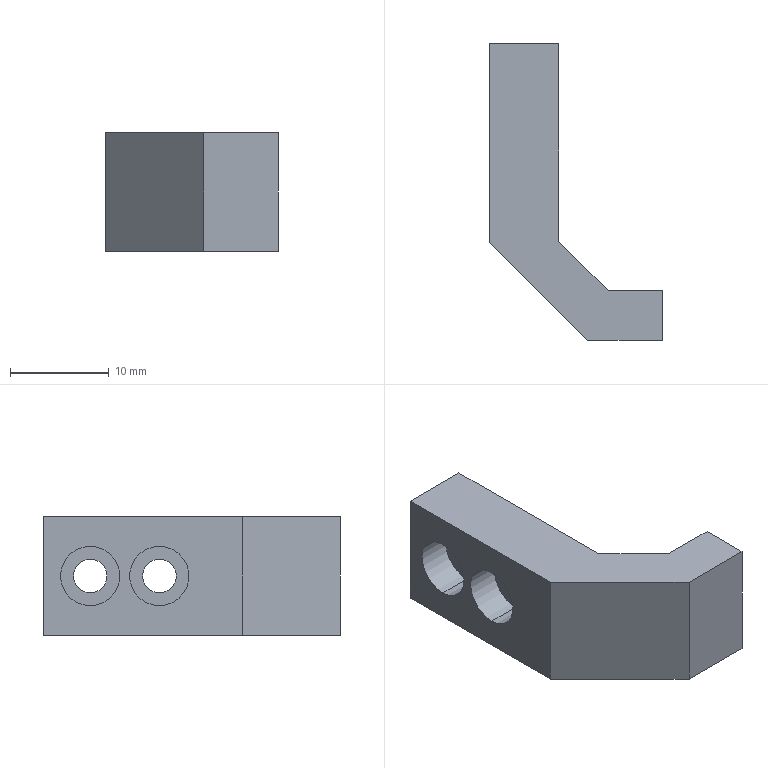Part | SolidWorks | features Extrusion 1, Fillet 1, HoleWzd 1, ICE 1 | 1 solid | 27 faces | box 17.5 x 30 x 12 mm | volume 2171 mm3 | plane 17 | cylinder 10 | commonest cylinder face diameters 3.4 x4 6 x4 4 x2
STEP:
#1=CARTESIAN_POINT('',(3.4,-4.7,-3.));
#2=VERTEX_POINT('',#1);
#3=CARTESIAN_POINT('',(3.4,-4.7,3.));
#4=VERTEX_POINT('',#3);
#5=CARTESIAN_POINT('',(3.4,-4.7,0.));
#6=DIRECTION('',(-1.,0.,0.));
#7=DIRECTION('',(0.,0.,1.));
#8=AXIS2_PLACEMENT_3D('',#5,#6,#7);
#9=CIRCLE('',#8,3.);
#10=EDGE_CURVE('',#2,#4,#9,.T.);
#11=ORIENTED_EDGE('',*,*,#10,.F.);
#12=CARTESIAN_POINT('',(0.,-4.7,-3.));
#13=VERTEX_POINT('',#12);
#14=CARTESIAN_POINT('',(0.,-4.7,-3.));
#15=DIRECTION('',(-1.,0.,0.));
#16=VECTOR('',#15,1000.);
#17=LINE('',#14,#16);
#18=EDGE_CURVE('',#2,#13,#17,.T.);
#19=ORIENTED_EDGE('',*,*,#18,.T.);
#20=CARTESIAN_POINT('',(0.,-4.7,3.));
#21=VERTEX_POINT('',#20);
#22=CARTESIAN_POINT('',(0.,-4.7,0.));
#23=DIRECTION('',(-1.,0.,0.));
#24=DIRECTION('',(0.,0.,1.));
#25=AXIS2_PLACEMENT_3D('',#22,#23,#24);
#26=CIRCLE('',#25,3.);
#27=EDGE_CURVE('',#13,#21,#26,.T.);
#28=ORIENTED_EDGE('',*,*,#27,.T.);
#29=CARTESIAN_POINT('',(0.,-4.7,3.));
#30=DIRECTION('',(-1.,0.,0.));
#31=VECTOR('',#30,1000.);
#32=LINE('',#29,#31);
#33=EDGE_CURVE('',#4,#21,#32,.T.);
#34=ORIENTED_EDGE('',*,*,#33,.F.);
#35=EDGE_LOOP('',(#11,#19,#28,#34));
#36=FACE_OUTER_BOUND('',#35,.T.);
#37=CARTESIAN_POINT('',(0.,-4.7,0.));
#38=DIRECTION('',(-1.,0.,0.));
#39=DIRECTION('',(0.,0.,1.));
#40=AXIS2_PLACEMENT_3D('',#37,#38,#39);
#41=CYLINDRICAL_SURFACE('',#40,3.);
#42=ADVANCED_FACE('',(#36),#41,.F.);
#43=CARTESIAN_POINT('',(5.,-4.7,-1.7));
#44=VERTEX_POINT('',#43);
#45=CARTESIAN_POINT('',(5.,-4.7,1.7));
#46=VERTEX_POINT('',#45);
#47=CARTESIAN_POINT('',(5.,-4.7,0.));
#48=DIRECTION('',(-1.,0.,0.));
#49=DIRECTION('',(0.,-1.,0.));
#50=AXIS2_PLACEMENT_3D('',#47,#48,#49);
#51=CIRCLE('',#50,1.7);
#52=EDGE_CURVE('',#44,#46,#51,.T.);
#53=ORIENTED_EDGE('',*,*,#52,.F.);
#54=CARTESIAN_POINT('',(3.4,-4.7,-1.7));
#55=VERTEX_POINT('',#54);
#56=CARTESIAN_POINT('',(0.,-4.7,-1.7));
#57=DIRECTION('',(-1.,0.,0.));
#58=VECTOR('',#57,1000.);
#59=LINE('',#56,#58);
#60=EDGE_CURVE('',#44,#55,#59,.T.);
#61=ORIENTED_EDGE('',*,*,#60,.T.);
#62=CARTESIAN_POINT('',(3.4,-4.7,1.7));
#63=VERTEX_POINT('',#62);
#64=CARTESIAN_POINT('',(3.4,-4.7,0.));
#65=DIRECTION('',(-1.,0.,0.));
#66=DIRECTION('',(0.,0.,1.));
#67=AXIS2_PLACEMENT_3D('',#64,#65,#66);
#68=CIRCLE('',#67,1.7);
#69=EDGE_CURVE('',#55,#63,#68,.T.);
#70=ORIENTED_EDGE('',*,*,#69,.T.);
#71=CARTESIAN_POINT('',(0.,-4.7,1.7));
#72=DIRECTION('',(-1.,0.,0.));
#73=VECTOR('',#72,1000.);
#74=LINE('',#71,#73);
#75=EDGE_CURVE('',#46,#63,#74,.T.);
#76=ORIENTED_EDGE('',*,*,#75,.F.);
#77=EDGE_LOOP('',(#53,#61,#70,#76));
#78=FACE_OUTER_BOUND('',#77,.T.);
#79=CARTESIAN_POINT('',(0.,-4.7,0.));
#80=DIRECTION('',(-1.,0.,0.));
#81=DIRECTION('',(0.,0.,1.));
#82=AXIS2_PLACEMENT_3D('',#79,#80,#81);
#83=CYLINDRICAL_SURFACE('',#82,1.7);
#84=ADVANCED_FACE('',(#78),#83,.F.);
#85=CARTESIAN_POINT('',(3.4,-11.7,-3.));
#86=VERTEX_POINT('',#85);
#87=CARTESIAN_POINT('',(3.4,-11.7,3.));
#88=VERTEX_POINT('',#87);
#89=CARTESIAN_POINT('',(3.4,-11.7,0.));
#90=DIRECTION('',(-1.,0.,0.));
#91=DIRECTION('',(0.,0.,1.));
#92=AXIS2_PLACEMENT_3D('',#89,#90,#91);
#93=CIRCLE('',#92,3.);
#94=EDGE_CURVE('',#86,#88,#93,.T.);
#95=ORIENTED_EDGE('',*,*,#94,.F.);
#96=CARTESIAN_POINT('',(0.,-11.7,-3.));
#97=VERTEX_POINT('',#96);
#98=CARTESIAN_POINT('',(0.,-11.7,-3.));
#99=DIRECTION('',(-1.,0.,0.));
#100=VECTOR('',#99,1000.);
#101=LINE('',#98,#100);
#102=EDGE_CURVE('',#86,#97,#101,.T.);
#103=ORIENTED_EDGE('',*,*,#102,.T.);
#104=CARTESIAN_POINT('',(0.,-11.7,3.));
#105=VERTEX_POINT('',#104);
#106=CARTESIAN_POINT('',(0.,-11.7,0.));
#107=DIRECTION('',(-1.,0.,0.));
#108=DIRECTION('',(0.,0.,1.));
#109=AXIS2_PLACEMENT_3D('',#106,#107,#108);
#110=CIRCLE('',#109,3.);
#111=EDGE_CURVE('',#97,#105,#110,.T.);
#112=ORIENTED_EDGE('',*,*,#111,.T.);
#113=CARTESIAN_POINT('',(0.,-11.7,3.));
#114=DIRECTION('',(-1.,0.,0.));
#115=VECTOR('',#114,1000.);
#116=LINE('',#113,#115);
#117=EDGE_CURVE('',#88,#105,#116,.T.);
#118=ORIENTED_EDGE('',*,*,#117,.F.);
#119=EDGE_LOOP('',(#95,#103,#112,#118));
#120=FACE_OUTER_BOUND('',#119,.T.);
#121=CARTESIAN_POINT('',(0.,-11.7,0.));
#122=DIRECTION('',(-1.,0.,0.));
#123=DIRECTION('',(0.,0.,1.));
#124=AXIS2_PLACEMENT_3D('',#121,#122,#123);
#125=CYLINDRICAL_SURFACE('',#124,3.);
#126=ADVANCED_FACE('',(#120),#125,.F.);
#127=CARTESIAN_POINT('',(5.,-11.7,-1.7));
#128=VERTEX_POINT('',#127);
#129=CARTESIAN_POINT('',(5.,-11.7,1.7));
#130=VERTEX_POINT('',#129);
#131=CARTESIAN_POINT('',(5.,-11.7,0.));
#132=DIRECTION('',(-1.,0.,0.));
#133=DIRECTION('',(0.,-1.,0.));
#134=AXIS2_PLACEMENT_3D('',#131,#132,#133);
#135=CIRCLE('',#134,1.7);
#136=EDGE_CURVE('',#128,#130,#135,.T.);
#137=ORIENTED_EDGE('',*,*,#136,.F.);
#138=CARTESIAN_POINT('',(3.4,-11.7,-1.7));
#139=VERTEX_POINT('',#138);
#140=CARTESIAN_POINT('',(0.,-11.7,-1.7));
#141=DIRECTION('',(-1.,0.,0.));
#142=VECTOR('',#141,1000.);
#143=LINE('',#140,#142);
#144=EDGE_CURVE('',#128,#139,#143,.T.);
#145=ORIENTED_EDGE('',*,*,#144,.T.);
#146=CARTESIAN_POINT('',(3.4,-11.7,1.7));
#147=VERTEX_POINT('',#146);
#148=CARTESIAN_POINT('',(3.4,-11.7,0.));
#149=DIRECTION('',(-1.,0.,0.));
#150=DIRECTION('',(0.,0.,1.));
#151=AXIS2_PLACEMENT_3D('',#148,#149,#150);
#152=CIRCLE('',#151,1.7);
#153=EDGE_CURVE('',#139,#147,#152,.T.);
#154=ORIENTED_EDGE('',*,*,#153,.T.);
#155=CARTESIAN_POINT('',(0.,-11.7,1.7));
#156=DIRECTION('',(-1.,0.,0.));
#157=VECTOR('',#156,1000.);
#158=LINE('',#155,#157);
#159=EDGE_CURVE('',#130,#147,#158,.T.);
#160=ORIENTED_EDGE('',*,*,#159,.F.);
#161=EDGE_LOOP('',(#137,#145,#154,#160));
#162=FACE_OUTER_BOUND('',#161,.T.);
#163=CARTESIAN_POINT('',(0.,-11.7,0.));
#164=DIRECTION('',(-1.,0.,0.));
#165=DIRECTION('',(0.,0.,1.));
#166=AXIS2_PLACEMENT_3D('',#163,#164,#165);
#167=CYLINDRICAL_SURFACE('',#166,1.7);
#168=ADVANCED_FACE('',(#162),#167,.F.);
#169=CARTESIAN_POINT('',(7.,-20.,6.));
#170=VERTEX_POINT('',#169);
#171=CARTESIAN_POINT('',(7.,-20.,2.));
#172=VERTEX_POINT('',#171);
#173=CARTESIAN_POINT('',(7.,-20.,6.));
#174=DIRECTION('',(0.,0.,-1.));
#175=VECTOR('',#174,1000.);
#176=LINE('',#173,#175);
#177=EDGE_CURVE('',#170,#172,#176,.T.);
#178=ORIENTED_EDGE('',*,*,#177,.T.);
#179=CARTESIAN_POINT('',(7.,-18.,4.));
#180=VERTEX_POINT('',#179);
#181=CARTESIAN_POINT('',(7.,-18.,2.));
#182=DIRECTION('',(-1.,0.,0.));
#183=DIRECTION('',(0.,-1.,0.));
#184=AXIS2_PLACEMENT_3D('',#181,#182,#183);
#185=CIRCLE('',#184,2.);
#186=EDGE_CURVE('',#172,#180,#185,.T.);
#187=ORIENTED_EDGE('',*,*,#186,.T.);
#188=CARTESIAN_POINT('',(7.,0.,4.));
#189=VERTEX_POINT('',#188);
#190=CARTESIAN_POINT('',(7.,-20.,4.));
#191=DIRECTION('',(0.,1.,0.));
#192=VECTOR('',#191,1000.);
#193=LINE('',#190,#192);
#194=EDGE_CURVE('',#180,#189,#193,.T.);
#195=ORIENTED_EDGE('',*,*,#194,.T.);
#196=CARTESIAN_POINT('',(7.,0.,6.));
#197=VERTEX_POINT('',#196);
#198=CARTESIAN_POINT('',(7.,0.,6.));
#199=DIRECTION('',(0.,0.,-1.));
#200=VECTOR('',#199,1000.);
#201=LINE('',#198,#200);
#202=EDGE_CURVE('',#197,#189,#201,.T.);
#203=ORIENTED_EDGE('',*,*,#202,.F.);
#204=CARTESIAN_POINT('',(7.,-20.,6.));
#205=DIRECTION('',(0.,1.,0.));
#206=VECTOR('',#205,1000.);
#207=LINE('',#204,#206);
#208=EDGE_CURVE('',#170,#197,#207,.T.);
#209=ORIENTED_EDGE('',*,*,#208,.F.);
#210=EDGE_LOOP('',(#178,#187,#195,#203,#209));
#211=FACE_OUTER_BOUND('',#210,.T.);
#212=CARTESIAN_POINT('',(7.,-20.,6.));
#213=DIRECTION('',(-1.,0.,0.));
#214=DIRECTION('',(0.,-1.,0.));
#215=AXIS2_PLACEMENT_3D('',#212,#213,#214);
#216=PLANE('',#215);
#217=ADVANCED_FACE('',(#211),#216,.F.);
#218=ORIENTED_EDGE('',*,*,#202,.T.);
#219=CARTESIAN_POINT('',(5.,0.,4.));
#220=VERTEX_POINT('',#219);
#221=CARTESIAN_POINT('',(7.,0.,4.));
#222=DIRECTION('',(1.,0.,0.));
#223=VECTOR('',#222,1000.);
#224=LINE('',#221,#223);
#225=EDGE_CURVE('',#220,#189,#224,.T.);
#226=ORIENTED_EDGE('',*,*,#225,.F.);
#227=CARTESIAN_POINT('',(5.,0.,-4.));
#228=VERTEX_POINT('',#227);
#229=CARTESIAN_POINT('',(5.,0.,-4.));
#230=DIRECTION('',(0.,0.,1.));
#231=VECTOR('',#230,1000.);
#232=LINE('',#229,#231);
#233=EDGE_CURVE('',#228,#220,#232,.T.);
#234=ORIENTED_EDGE('',*,*,#233,.F.);
#235=CARTESIAN_POINT('',(7.,0.,-4.));
#236=VERTEX_POINT('',#235);
#237=CARTESIAN_POINT('',(7.,0.,-4.));
#238=DIRECTION('',(-1.,0.,0.));
#239=VECTOR('',#238,1000.);
#240=LINE('',#237,#239);
#241=EDGE_CURVE('',#236,#228,#240,.T.);
#242=ORIENTED_EDGE('',*,*,#241,.F.);
#243=CARTESIAN_POINT('',(7.,0.,-6.));
#244=VERTEX_POINT('',#243);
#245=CARTESIAN_POINT('',(7.,0.,6.));
#246=DIRECTION('',(0.,0.,-1.));
#247=VECTOR('',#246,1000.);
#248=LINE('',#245,#247);
#249=EDGE_CURVE('',#236,#244,#248,.T.);
#250=ORIENTED_EDGE('',*,*,#249,.T.);
#251=CARTESIAN_POINT('',(0.,0.,-6.));
#252=VERTEX_POINT('',#251);
#253=CARTESIAN_POINT('',(7.,0.,-6.));
#254=DIRECTION('',(-1.,0.,0.));
#255=VECTOR('',#254,1000.);
#256=LINE('',#253,#255);
#257=EDGE_CURVE('',#244,#252,#256,.T.);
#258=ORIENTED_EDGE('',*,*,#257,.T.);
#259=CARTESIAN_POINT('',(0.,0.,6.));
#260=VERTEX_POINT('',#259);
#261=CARTESIAN_POINT('',(0.,0.,6.));
#262=DIRECTION('',(0.,0.,-1.));
#263=VECTOR('',#262,1000.);
#264=LINE('',#261,#263);
#265=EDGE_CURVE('',#260,#252,#264,.T.);
#266=ORIENTED_EDGE('',*,*,#265,.F.);
#267=CARTESIAN_POINT('',(7.,0.,6.));
#268=DIRECTION('',(-1.,0.,0.));
#269=VECTOR('',#268,1000.);
#270=LINE('',#267,#269);
#271=EDGE_CURVE('',#197,#260,#270,.T.);
#272=ORIENTED_EDGE('',*,*,#271,.F.);
#273=EDGE_LOOP('',(#218,#226,#234,#242,#250,#258,#266,#272));
#274=FACE_OUTER_BOUND('',#273,.T.);
#275=CARTESIAN_POINT('',(7.,0.,6.));
#276=DIRECTION('',(0.,-1.,0.));
#277=DIRECTION('',(1.,0.,0.));
#278=AXIS2_PLACEMENT_3D('',#275,#276,#277);
#279=PLANE('',#278);
#280=ADVANCED_FACE('',(#274),#279,.F.);
#281=CARTESIAN_POINT('',(0.,-4.7,0.));
#282=DIRECTION('',(-1.,0.,0.));
#283=DIRECTION('',(0.,0.,1.));
#284=AXIS2_PLACEMENT_3D('',#281,#282,#283);
#285=CIRCLE('',#284,3.);
#286=EDGE_CURVE('',#21,#13,#285,.T.);
#287=ORIENTED_EDGE('',*,*,#286,.F.);
#288=ORIENTED_EDGE('',*,*,#27,.F.);
#289=EDGE_LOOP('',(#287,#288));
#290=FACE_BOUND('',#289,.T.);
#291=CARTESIAN_POINT('',(0.,-11.7,0.));
#292=DIRECTION('',(-1.,0.,0.));
#293=DIRECTION('',(0.,0.,1.));
#294=AXIS2_PLACEMENT_3D('',#291,#292,#293);
#295=CIRCLE('',#294,3.);
#296=EDGE_CURVE('',#105,#97,#295,.T.);
#297=ORIENTED_EDGE('',*,*,#296,.F.);
#298=ORIENTED_EDGE('',*,*,#111,.F.);
#299=EDGE_LOOP('',(#297,#298));
#300=FACE_BOUND('',#299,.T.);
#301=CARTESIAN_POINT('',(0.,-20.071,-6.));
#302=VERTEX_POINT('',#301);
#303=CARTESIAN_POINT('',(0.,0.,-6.));
#304=DIRECTION('',(0.,-1.,0.));
#305=VECTOR('',#304,1000.);
#306=LINE('',#303,#305);
#307=EDGE_CURVE('',#252,#302,#306,.T.);
#308=ORIENTED_EDGE('',*,*,#307,.T.);
#309=CARTESIAN_POINT('',(0.,-20.071,6.));
#310=VERTEX_POINT('',#309);
#311=CARTESIAN_POINT('',(0.,-20.071,6.));
#312=DIRECTION('',(0.,0.,-1.));
#313=VECTOR('',#312,1000.);
#314=LINE('',#311,#313);
#315=EDGE_CURVE('',#310,#302,#314,.T.);
#316=ORIENTED_EDGE('',*,*,#315,.F.);
#317=CARTESIAN_POINT('',(0.,0.,6.));
#318=DIRECTION('',(0.,-1.,0.));
#319=VECTOR('',#318,1000.);
#320=LINE('',#317,#319);
#321=EDGE_CURVE('',#260,#310,#320,.T.);
#322=ORIENTED_EDGE('',*,*,#321,.F.);
#323=ORIENTED_EDGE('',*,*,#265,.T.);
#324=EDGE_LOOP('',(#308,#316,#322,#323));
#325=FACE_OUTER_BOUND('',#324,.T.);
#326=CARTESIAN_POINT('',(0.,0.,6.));
#327=DIRECTION('',(1.,0.,0.));
#328=DIRECTION('',(0.,1.,0.));
#329=AXIS2_PLACEMENT_3D('',#326,#327,#328);
#330=PLANE('',#329);
#331=ADVANCED_FACE('',(#290,#300,#325),#330,.F.);
#332=CARTESIAN_POINT('',(9.929,-30.,-6.));
#333=VERTEX_POINT('',#332);
#334=CARTESIAN_POINT('',(0.,-20.071,-6.));
#335=DIRECTION('',(0.7071,-0.7071,0.));
#336=VECTOR('',#335,1000.);
#337=LINE('',#334,#336);
#338=EDGE_CURVE('',#302,#333,#337,.T.);
#339=ORIENTED_EDGE('',*,*,#338,.T.);
#340=CARTESIAN_POINT('',(9.929,-30.,6.));
#341=VERTEX_POINT('',#340);
#342=CARTESIAN_POINT('',(9.929,-30.,6.));
#343=DIRECTION('',(0.,0.,-1.));
#344=VECTOR('',#343,1000.);
#345=LINE('',#342,#344);
#346=EDGE_CURVE('',#341,#333,#345,.T.);
#347=ORIENTED_EDGE('',*,*,#346,.F.);
#348=CARTESIAN_POINT('',(0.,-20.071,6.));
#349=DIRECTION('',(0.7071,-0.7071,0.));
#350=VECTOR('',#349,1000.);
#351=LINE('',#348,#350);
#352=EDGE_CURVE('',#310,#341,#351,.T.);
#353=ORIENTED_EDGE('',*,*,#352,.F.);
#354=ORIENTED_EDGE('',*,*,#315,.T.);
#355=EDGE_LOOP('',(#339,#347,#353,#354));
#356=FACE_OUTER_BOUND('',#355,.T.);
#357=CARTESIAN_POINT('',(0.,-20.071,6.));
#358=DIRECTION('',(0.7071,0.7071,0.));
#359=DIRECTION('',(-0.7071,0.7071,0.));
#360=AXIS2_PLACEMENT_3D('',#357,#358,#359);
#361=PLANE('',#360);
#362=ADVANCED_FACE('',(#356),#361,.F.);
#363=CARTESIAN_POINT('',(17.5,-30.,-6.));
#364=VERTEX_POINT('',#363);
#365=CARTESIAN_POINT('',(17.5,-30.,-6.));
#366=DIRECTION('',(1.,0.,0.));
#367=VECTOR('',#366,1000.);
#368=LINE('',#365,#367);
#369=EDGE_CURVE('',#333,#364,#368,.T.);
#370=ORIENTED_EDGE('',*,*,#369,.T.);
#371=CARTESIAN_POINT('',(17.5,-30.,6.));
#372=VERTEX_POINT('',#371);
#373=CARTESIAN_POINT('',(17.5,-30.,6.));
#374=DIRECTION('',(0.,0.,-1.));
#375=VECTOR('',#374,1000.);
#376=LINE('',#373,#375);
#377=EDGE_CURVE('',#372,#364,#376,.T.);
#378=ORIENTED_EDGE('',*,*,#377,.F.);
#379=CARTESIAN_POINT('',(17.5,-30.,6.));
#380=DIRECTION('',(1.,0.,0.));
#381=VECTOR('',#380,1000.);
#382=LINE('',#379,#381);
#383=EDGE_CURVE('',#341,#372,#382,.T.);
#384=ORIENTED_EDGE('',*,*,#383,.F.);
#385=ORIENTED_EDGE('',*,*,#346,.T.);
#386=EDGE_LOOP('',(#370,#378,#384,#385));
#387=FACE_OUTER_BOUND('',#386,.T.);
#388=CARTESIAN_POINT('',(17.5,-30.,6.));
#389=DIRECTION('',(0.,1.,0.));
#390=DIRECTION('',(-1.,0.,0.));
#391=AXIS2_PLACEMENT_3D('',#388,#389,#390);
#392=PLANE('',#391);
#393=ADVANCED_FACE('',(#387),#392,.F.);
#394=CARTESIAN_POINT('',(17.5,-25.,-6.));
#395=VERTEX_POINT('',#394);
#396=CARTESIAN_POINT('',(17.5,-25.,-6.));
#397=DIRECTION('',(0.,1.,0.));
#398=VECTOR('',#397,1000.);
#399=LINE('',#396,#398);
#400=EDGE_CURVE('',#364,#395,#399,.T.);
#401=ORIENTED_EDGE('',*,*,#400,.T.);
#402=CARTESIAN_POINT('',(17.5,-25.,6.));
#403=VERTEX_POINT('',#402);
#404=CARTESIAN_POINT('',(17.5,-25.,6.));
#405=DIRECTION('',(0.,0.,-1.));
#406=VECTOR('',#405,1000.);
#407=LINE('',#404,#406);
#408=EDGE_CURVE('',#403,#395,#407,.T.);
#409=ORIENTED_EDGE('',*,*,#408,.F.);
#410=CARTESIAN_POINT('',(17.5,-25.,6.));
#411=DIRECTION('',(0.,1.,0.));
#412=VECTOR('',#411,1000.);
#413=LINE('',#410,#412);
#414=EDGE_CURVE('',#372,#403,#413,.T.);
#415=ORIENTED_EDGE('',*,*,#414,.F.);
#416=ORIENTED_EDGE('',*,*,#377,.T.);
#417=EDGE_LOOP('',(#401,#409,#415,#416));
#418=FACE_OUTER_BOUND('',#417,.T.);
#419=CARTESIAN_POINT('',(17.5,-25.,6.));
#420=DIRECTION('',(-1.,0.,0.));
#421=DIRECTION('',(0.,0.,1.));
#422=AXIS2_PLACEMENT_3D('',#419,#420,#421);
#423=PLANE('',#422);
#424=ADVANCED_FACE('',(#418),#423,.F.);
#425=CARTESIAN_POINT('',(12.,-25.,-6.));
#426=VERTEX_POINT('',#425);
#427=CARTESIAN_POINT('',(12.,-25.,-6.));
#428=DIRECTION('',(-1.,0.,0.));
#429=VECTOR('',#428,1000.);
#430=LINE('',#427,#429);
#431=EDGE_CURVE('',#395,#426,#430,.T.);
#432=ORIENTED_EDGE('',*,*,#431,.T.);
#433=CARTESIAN_POINT('',(12.,-25.,6.));
#434=VERTEX_POINT('',#433);
#435=CARTESIAN_POINT('',(12.,-25.,6.));
#436=DIRECTION('',(0.,0.,-1.));
#437=VECTOR('',#436,1000.);
#438=LINE('',#435,#437);
#439=EDGE_CURVE('',#434,#426,#438,.T.);
#440=ORIENTED_EDGE('',*,*,#439,.F.);
#441=CARTESIAN_POINT('',(12.,-25.,6.));
#442=DIRECTION('',(-1.,0.,0.));
#443=VECTOR('',#442,1000.);
#444=LINE('',#441,#443);
#445=EDGE_CURVE('',#403,#434,#444,.T.);
#446=ORIENTED_EDGE('',*,*,#445,.F.);
#447=ORIENTED_EDGE('',*,*,#408,.T.);
#448=EDGE_LOOP('',(#432,#440,#446,#447));
#449=FACE_OUTER_BOUND('',#448,.T.);
#450=CARTESIAN_POINT('',(12.,-25.,6.));
#451=DIRECTION('',(0.,-1.,0.));
#452=DIRECTION('',(1.,0.,0.));
#453=AXIS2_PLACEMENT_3D('',#450,#451,#452);
#454=PLANE('',#453);
#455=ADVANCED_FACE('',(#449),#454,.F.);
#456=CARTESIAN_POINT('',(7.,-20.,-6.));
#457=VERTEX_POINT('',#456);
#458=CARTESIAN_POINT('',(12.,-25.,-6.));
#459=DIRECTION('',(-0.7071,0.7071,0.));
#460=VECTOR('',#459,1000.);
#461=LINE('',#458,#460);
#462=EDGE_CURVE('',#426,#457,#461,.T.);
#463=ORIENTED_EDGE('',*,*,#462,.T.);
#464=CARTESIAN_POINT('',(7.,-20.,-2.));
#465=VERTEX_POINT('',#464);
#466=CARTESIAN_POINT('',(7.,-20.,6.));
#467=DIRECTION('',(0.,0.,-1.));
#468=VECTOR('',#467,1000.);
#469=LINE('',#466,#468);
#470=EDGE_CURVE('',#465,#457,#469,.T.);
#471=ORIENTED_EDGE('',*,*,#470,.F.);
#472=CARTESIAN_POINT('',(7.,-20.,-4.));
#473=DIRECTION('',(0.,0.,-1.));
#474=VECTOR('',#473,1000.);
#475=LINE('',#472,#474);
#476=EDGE_CURVE('',#172,#465,#475,.T.);
#477=ORIENTED_EDGE('',*,*,#476,.F.);
#478=ORIENTED_EDGE('',*,*,#177,.F.);
#479=CARTESIAN_POINT('',(12.,-25.,6.));
#480=DIRECTION('',(-0.7071,0.7071,0.));
#481=VECTOR('',#480,1000.);
#482=LINE('',#479,#481);
#483=EDGE_CURVE('',#434,#170,#482,.T.);
#484=ORIENTED_EDGE('',*,*,#483,.F.);
#485=ORIENTED_EDGE('',*,*,#439,.T.);
#486=EDGE_LOOP('',(#463,#471,#477,#478,#484,#485));
#487=FACE_OUTER_BOUND('',#486,.T.);
#488=CARTESIAN_POINT('',(12.,-25.,6.));
#489=DIRECTION('',(-0.7071,-0.7071,0.));
#490=DIRECTION('',(0.7071,-0.7071,0.));
#491=AXIS2_PLACEMENT_3D('',#488,#489,#490);
#492=PLANE('',#491);
#493=ADVANCED_FACE('',(#487),#492,.F.);
#494=ORIENTED_EDGE('',*,*,#249,.F.);
#495=CARTESIAN_POINT('',(7.,-18.,-4.));
#496=VERTEX_POINT('',#495);
#497=CARTESIAN_POINT('',(7.,-20.,-4.));
#498=DIRECTION('',(0.,1.,0.));
#499=VECTOR('',#498,1000.);
#500=LINE('',#497,#499);
#501=EDGE_CURVE('',#496,#236,#500,.T.);
#502=ORIENTED_EDGE('',*,*,#501,.F.);
#503=CARTESIAN_POINT('',(7.,-18.,-2.));
#504=DIRECTION('',(-1.,0.,0.));
#505=DIRECTION('',(0.,-1.,0.));
#506=AXIS2_PLACEMENT_3D('',#503,#504,#505);
#507=CIRCLE('',#506,2.);
#508=EDGE_CURVE('',#496,#465,#507,.T.);
#509=ORIENTED_EDGE('',*,*,#508,.T.);
#510=ORIENTED_EDGE('',*,*,#470,.T.);
#511=CARTESIAN_POINT('',(7.,-20.,-6.));
#512=DIRECTION('',(0.,1.,0.));
#513=VECTOR('',#512,1000.);
#514=LINE('',#511,#513);
#515=EDGE_CURVE('',#457,#244,#514,.T.);
#516=ORIENTED_EDGE('',*,*,#515,.T.);
#517=EDGE_LOOP('',(#494,#502,#509,#510,#516));
#518=FACE_OUTER_BOUND('',#517,.T.);
#519=CARTESIAN_POINT('',(7.,-20.,6.));
#520=DIRECTION('',(-1.,0.,0.));
#521=DIRECTION('',(0.,-1.,0.));
#522=AXIS2_PLACEMENT_3D('',#519,#520,#521);
#523=PLANE('',#522);
#524=ADVANCED_FACE('',(#518),#523,.F.);
#525=ORIENTED_EDGE('',*,*,#271,.T.);
#526=ORIENTED_EDGE('',*,*,#321,.T.);
#527=ORIENTED_EDGE('',*,*,#352,.T.);
#528=ORIENTED_EDGE('',*,*,#383,.T.);
#529=ORIENTED_EDGE('',*,*,#414,.T.);
#530=ORIENTED_EDGE('',*,*,#445,.T.);
#531=ORIENTED_EDGE('',*,*,#483,.T.);
#532=ORIENTED_EDGE('',*,*,#208,.T.);
#533=EDGE_LOOP('',(#525,#526,#527,#528,#529,#530,#531,#532));
#534=FACE_OUTER_BOUND('',#533,.T.);
#535=CARTESIAN_POINT('',(0.,0.,6.));
#536=DIRECTION('',(0.,0.,1.));
#537=DIRECTION('',(1.,0.,0.));
#538=AXIS2_PLACEMENT_3D('',#535,#536,#537);
#539=PLANE('',#538);
#540=ADVANCED_FACE('',(#534),#539,.T.);
#541=ORIENTED_EDGE('',*,*,#257,.F.);
#542=ORIENTED_EDGE('',*,*,#515,.F.);
#543=ORIENTED_EDGE('',*,*,#462,.F.);
#544=ORIENTED_EDGE('',*,*,#431,.F.);
#545=ORIENTED_EDGE('',*,*,#400,.F.);
#546=ORIENTED_EDGE('',*,*,#369,.F.);
#547=ORIENTED_EDGE('',*,*,#338,.F.);
#548=ORIENTED_EDGE('',*,*,#307,.F.);
#549=EDGE_LOOP('',(#541,#542,#543,#544,#545,#546,#547,#548));
#550=FACE_OUTER_BOUND('',#549,.T.);
#551=CARTESIAN_POINT('',(0.,0.,-6.));
#552=DIRECTION('',(0.,0.,1.));
#553=DIRECTION('',(1.,0.,0.));
#554=AXIS2_PLACEMENT_3D('',#551,#552,#553);
#555=PLANE('',#554);
#556=ADVANCED_FACE('',(#550),#555,.F.);
#557=ORIENTED_EDGE('',*,*,#194,.F.);
#558=CARTESIAN_POINT('',(5.,-18.,4.));
#559=VERTEX_POINT('',#558);
#560=CARTESIAN_POINT('',(5.,-18.,4.));
#561=DIRECTION('',(-1.,0.,0.));
#562=VECTOR('',#561,1000.);
#563=LINE('',#560,#562);
#564=EDGE_CURVE('',#180,#559,#563,.T.);
#565=ORIENTED_EDGE('',*,*,#564,.T.);
#566=CARTESIAN_POINT('',(5.,-20.,4.));
#567=DIRECTION('',(0.,1.,0.));
#568=VECTOR('',#567,1000.);
#569=LINE('',#566,#568);
#570=EDGE_CURVE('',#559,#220,#569,.T.);
#571=ORIENTED_EDGE('',*,*,#570,.T.);
#572=ORIENTED_EDGE('',*,*,#225,.T.);
#573=EDGE_LOOP('',(#557,#565,#571,#572));
#574=FACE_OUTER_BOUND('',#573,.T.);
#575=CARTESIAN_POINT('',(7.,-20.,4.));
#576=DIRECTION('',(0.,0.,1.));
#577=DIRECTION('',(1.,0.,0.));
#578=AXIS2_PLACEMENT_3D('',#575,#576,#577);
#579=PLANE('',#578);
#580=ADVANCED_FACE('',(#574),#579,.F.);
#581=CARTESIAN_POINT('',(5.,-4.7,0.));
#582=DIRECTION('',(-1.,0.,0.));
#583=DIRECTION('',(0.,-1.,0.));
#584=AXIS2_PLACEMENT_3D('',#581,#582,#583);
#585=CIRCLE('',#584,1.7);
#586=EDGE_CURVE('',#46,#44,#585,.T.);
#587=ORIENTED_EDGE('',*,*,#586,.T.);
#588=ORIENTED_EDGE('',*,*,#52,.T.);
#589=EDGE_LOOP('',(#587,#588));
#590=FACE_BOUND('',#589,.T.);
#591=CARTESIAN_POINT('',(5.,-11.7,0.));
#592=DIRECTION('',(-1.,0.,0.));
#593=DIRECTION('',(0.,-1.,0.));
#594=AXIS2_PLACEMENT_3D('',#591,#592,#593);
#595=CIRCLE('',#594,1.7);
#596=EDGE_CURVE('',#130,#128,#595,.T.);
#597=ORIENTED_EDGE('',*,*,#596,.T.);
#598=ORIENTED_EDGE('',*,*,#136,.T.);
#599=EDGE_LOOP('',(#597,#598));
#600=FACE_BOUND('',#599,.T.);
#601=ORIENTED_EDGE('',*,*,#570,.F.);
#602=CARTESIAN_POINT('',(5.,-20.,2.));
#603=VERTEX_POINT('',#602);
#604=CARTESIAN_POINT('',(5.,-18.,2.));
#605=DIRECTION('',(1.,0.,0.));
#606=DIRECTION('',(0.,-1.,0.));
#607=AXIS2_PLACEMENT_3D('',#604,#605,#606);
#608=CIRCLE('',#607,2.);
#609=EDGE_CURVE('',#559,#603,#608,.T.);
#610=ORIENTED_EDGE('',*,*,#609,.T.);
#611=CARTESIAN_POINT('',(5.,-20.,-2.));
#612=VERTEX_POINT('',#611);
#613=CARTESIAN_POINT('',(5.,-20.,-4.));
#614=DIRECTION('',(0.,0.,1.));
#615=VECTOR('',#614,1000.);
#616=LINE('',#613,#615);
#617=EDGE_CURVE('',#612,#603,#616,.T.);
#618=ORIENTED_EDGE('',*,*,#617,.F.);
#619=CARTESIAN_POINT('',(5.,-18.,-4.));
#620=VERTEX_POINT('',#619);
#621=CARTESIAN_POINT('',(5.,-18.,-2.));
#622=DIRECTION('',(1.,0.,0.));
#623=DIRECTION('',(0.,-1.,0.));
#624=AXIS2_PLACEMENT_3D('',#621,#622,#623);
#625=CIRCLE('',#624,2.);
#626=EDGE_CURVE('',#612,#620,#625,.T.);
#627=ORIENTED_EDGE('',*,*,#626,.T.);
#628=CARTESIAN_POINT('',(5.,-20.,-4.));
#629=DIRECTION('',(0.,1.,0.));
#630=VECTOR('',#629,1000.);
#631=LINE('',#628,#630);
#632=EDGE_CURVE('',#620,#228,#631,.T.);
#633=ORIENTED_EDGE('',*,*,#632,.T.);
#634=ORIENTED_EDGE('',*,*,#233,.T.);
#635=EDGE_LOOP('',(#601,#610,#618,#627,#633,#634));
#636=FACE_OUTER_BOUND('',#635,.T.);
#637=CARTESIAN_POINT('',(5.,-20.,-4.));
#638=DIRECTION('',(-1.,0.,0.));
#639=DIRECTION('',(0.,-1.,0.));
#640=AXIS2_PLACEMENT_3D('',#637,#638,#639);
#641=PLANE('',#640);
#642=ADVANCED_FACE('',(#590,#600,#636),#641,.F.);
#643=ORIENTED_EDGE('',*,*,#632,.F.);
#644=CARTESIAN_POINT('',(7.,-18.,-4.));
#645=DIRECTION('',(1.,0.,0.));
#646=VECTOR('',#645,1000.);
#647=LINE('',#644,#646);
#648=EDGE_CURVE('',#620,#496,#647,.T.);
#649=ORIENTED_EDGE('',*,*,#648,.T.);
#650=ORIENTED_EDGE('',*,*,#501,.T.);
#651=ORIENTED_EDGE('',*,*,#241,.T.);
#652=EDGE_LOOP('',(#643,#649,#650,#651));
#653=FACE_OUTER_BOUND('',#652,.T.);
#654=CARTESIAN_POINT('',(7.,-20.,-4.));
#655=DIRECTION('',(0.,0.,-1.));
#656=DIRECTION('',(-1.,0.,0.));
#657=AXIS2_PLACEMENT_3D('',#654,#655,#656);
#658=PLANE('',#657);
#659=ADVANCED_FACE('',(#653),#658,.F.);
#660=ORIENTED_EDGE('',*,*,#617,.T.);
#661=CARTESIAN_POINT('',(7.,-20.,2.));
#662=DIRECTION('',(1.,0.,0.));
#663=VECTOR('',#662,1000.);
#664=LINE('',#661,#663);
#665=EDGE_CURVE('',#603,#172,#664,.T.);
#666=ORIENTED_EDGE('',*,*,#665,.T.);
#667=ORIENTED_EDGE('',*,*,#476,.T.);
#668=CARTESIAN_POINT('',(5.,-20.,-2.));
#669=DIRECTION('',(-1.,0.,0.));
#670=VECTOR('',#669,1000.);
#671=LINE('',#668,#670);
#672=EDGE_CURVE('',#465,#612,#671,.T.);
#673=ORIENTED_EDGE('',*,*,#672,.T.);
#674=EDGE_LOOP('',(#660,#666,#667,#673));
#675=FACE_OUTER_BOUND('',#674,.T.);
#676=CARTESIAN_POINT('',(0.,-20.,0.));
#677=DIRECTION('',(0.,-1.,0.));
#678=DIRECTION('',(1.,0.,0.));
#679=AXIS2_PLACEMENT_3D('',#676,#677,#678);
#680=PLANE('',#679);
#681=ADVANCED_FACE('',(#675),#680,.F.);
#682=ORIENTED_EDGE('',*,*,#609,.F.);
#683=ORIENTED_EDGE('',*,*,#564,.F.);
#684=ORIENTED_EDGE('',*,*,#186,.F.);
#685=ORIENTED_EDGE('',*,*,#665,.F.);
#686=EDGE_LOOP('',(#682,#683,#684,#685));
#687=FACE_OUTER_BOUND('',#686,.T.);
#688=CARTESIAN_POINT('',(0.,-18.,2.));
#689=DIRECTION('',(-1.,0.,0.));
#690=DIRECTION('',(0.,-1.,0.));
#691=AXIS2_PLACEMENT_3D('',#688,#689,#690);
#692=CYLINDRICAL_SURFACE('',#691,2.);
#693=ADVANCED_FACE('',(#687),#692,.F.);
#694=ORIENTED_EDGE('',*,*,#508,.F.);
#695=ORIENTED_EDGE('',*,*,#648,.F.);
#696=ORIENTED_EDGE('',*,*,#626,.F.);
#697=ORIENTED_EDGE('',*,*,#672,.F.);
#698=EDGE_LOOP('',(#694,#695,#696,#697));
#699=FACE_OUTER_BOUND('',#698,.T.);
#700=CARTESIAN_POINT('',(0.,-18.,-2.));
#701=DIRECTION('',(1.,0.,0.));
#702=DIRECTION('',(0.,1.,0.));
#703=AXIS2_PLACEMENT_3D('',#700,#701,#702);
#704=CYLINDRICAL_SURFACE('',#703,2.);
#705=ADVANCED_FACE('',(#699),#704,.F.);
#706=ORIENTED_EDGE('',*,*,#144,.F.);
#707=ORIENTED_EDGE('',*,*,#596,.F.);
#708=ORIENTED_EDGE('',*,*,#159,.T.);
#709=CARTESIAN_POINT('',(3.4,-11.7,0.));
#710=DIRECTION('',(-1.,0.,0.));
#711=DIRECTION('',(0.,0.,1.));
#712=AXIS2_PLACEMENT_3D('',#709,#710,#711);
#713=CIRCLE('',#712,1.7);
#714=EDGE_CURVE('',#147,#139,#713,.T.);
#715=ORIENTED_EDGE('',*,*,#714,.T.);
#716=EDGE_LOOP('',(#706,#707,#708,#715));
#717=FACE_OUTER_BOUND('',#716,.T.);
#718=CARTESIAN_POINT('',(0.,-11.7,0.));
#719=DIRECTION('',(-1.,0.,0.));
#720=DIRECTION('',(0.,0.,1.));
#721=AXIS2_PLACEMENT_3D('',#718,#719,#720);
#722=CYLINDRICAL_SURFACE('',#721,1.7);
#723=ADVANCED_FACE('',(#717),#722,.F.);
#724=ORIENTED_EDGE('',*,*,#714,.F.);
#725=ORIENTED_EDGE('',*,*,#153,.F.);
#726=EDGE_LOOP('',(#724,#725));
#727=FACE_BOUND('',#726,.T.);
#728=CARTESIAN_POINT('',(3.4,-11.7,0.));
#729=DIRECTION('',(-1.,0.,0.));
#730=DIRECTION('',(0.,0.,1.));
#731=AXIS2_PLACEMENT_3D('',#728,#729,#730);
#732=CIRCLE('',#731,3.);
#733=EDGE_CURVE('',#88,#86,#732,.T.);
#734=ORIENTED_EDGE('',*,*,#733,.T.);
#735=ORIENTED_EDGE('',*,*,#94,.T.);
#736=EDGE_LOOP('',(#734,#735));
#737=FACE_OUTER_BOUND('',#736,.T.);
#738=CARTESIAN_POINT('',(3.4,-10.,0.));
#739=DIRECTION('',(1.,0.,0.));
#740=DIRECTION('',(0.,0.,-1.));
#741=AXIS2_PLACEMENT_3D('',#738,#739,#740);
#742=PLANE('',#741);
#743=ADVANCED_FACE('',(#727,#737),#742,.F.);
#744=ORIENTED_EDGE('',*,*,#102,.F.);
#745=ORIENTED_EDGE('',*,*,#733,.F.);
#746=ORIENTED_EDGE('',*,*,#117,.T.);
#747=ORIENTED_EDGE('',*,*,#296,.T.);
#748=EDGE_LOOP('',(#744,#745,#746,#747));
#749=FACE_OUTER_BOUND('',#748,.T.);
#750=CARTESIAN_POINT('',(0.,-11.7,0.));
#751=DIRECTION('',(-1.,0.,0.));
#752=DIRECTION('',(0.,0.,1.));
#753=AXIS2_PLACEMENT_3D('',#750,#751,#752);
#754=CYLINDRICAL_SURFACE('',#753,3.);
#755=ADVANCED_FACE('',(#749),#754,.F.);
#756=ORIENTED_EDGE('',*,*,#60,.F.);
#757=ORIENTED_EDGE('',*,*,#586,.F.);
#758=ORIENTED_EDGE('',*,*,#75,.T.);
#759=CARTESIAN_POINT('',(3.4,-4.7,0.));
#760=DIRECTION('',(-1.,0.,0.));
#761=DIRECTION('',(0.,0.,1.));
#762=AXIS2_PLACEMENT_3D('',#759,#760,#761);
#763=CIRCLE('',#762,1.7);
#764=EDGE_CURVE('',#63,#55,#763,.T.);
#765=ORIENTED_EDGE('',*,*,#764,.T.);
#766=EDGE_LOOP('',(#756,#757,#758,#765));
#767=FACE_OUTER_BOUND('',#766,.T.);
#768=CARTESIAN_POINT('',(0.,-4.7,0.));
#769=DIRECTION('',(-1.,0.,0.));
#770=DIRECTION('',(0.,0.,1.));
#771=AXIS2_PLACEMENT_3D('',#768,#769,#770);
#772=CYLINDRICAL_SURFACE('',#771,1.7);
#773=ADVANCED_FACE('',(#767),#772,.F.);
#774=ORIENTED_EDGE('',*,*,#764,.F.);
#775=ORIENTED_EDGE('',*,*,#69,.F.);
#776=EDGE_LOOP('',(#774,#775));
#777=FACE_BOUND('',#776,.T.);
#778=CARTESIAN_POINT('',(3.4,-4.7,0.));
#779=DIRECTION('',(-1.,0.,0.));
#780=DIRECTION('',(0.,0.,1.));
#781=AXIS2_PLACEMENT_3D('',#778,#779,#780);
#782=CIRCLE('',#781,3.);
#783=EDGE_CURVE('',#4,#2,#782,.T.);
#784=ORIENTED_EDGE('',*,*,#783,.T.);
#785=ORIENTED_EDGE('',*,*,#10,.T.);
#786=EDGE_LOOP('',(#784,#785));
#787=FACE_OUTER_BOUND('',#786,.T.);
#788=CARTESIAN_POINT('',(3.4,-3.,0.));
#789=DIRECTION('',(1.,0.,0.));
#790=DIRECTION('',(0.,0.,-1.));
#791=AXIS2_PLACEMENT_3D('',#788,#789,#790);
#792=PLANE('',#791);
#793=ADVANCED_FACE('',(#777,#787),#792,.F.);
#794=ORIENTED_EDGE('',*,*,#18,.F.);
#795=ORIENTED_EDGE('',*,*,#783,.F.);
#796=ORIENTED_EDGE('',*,*,#33,.T.);
#797=ORIENTED_EDGE('',*,*,#286,.T.);
#798=EDGE_LOOP('',(#794,#795,#796,#797));
#799=FACE_OUTER_BOUND('',#798,.T.);
#800=CARTESIAN_POINT('',(0.,-4.7,0.));
#801=DIRECTION('',(-1.,0.,0.));
#802=DIRECTION('',(0.,0.,1.));
#803=AXIS2_PLACEMENT_3D('',#800,#801,#802);
#804=CYLINDRICAL_SURFACE('',#803,3.);
#805=ADVANCED_FACE('',(#799),#804,.F.);
#806=CLOSED_SHELL('',(#42,#84,#126,#168,#217,#280,#331,#362,#393,#424,#455,#493,#524,#540,#556,#580,#642,#659,#681,#693,#705,#723,#743,#755,#773,#793,#805));
#807=MANIFOLD_SOLID_BREP('',#806);
#808=CARTESIAN_POINT('',(0.,0.,0.));
#809=DIRECTION('',(0.,0.,1.));
#810=DIRECTION('',(1.,0.,0.));
#811=AXIS2_PLACEMENT_3D('',#808,#809,#810);
#812=(LENGTH_UNIT()NAMED_UNIT(*)SI_UNIT(.MILLI.,.METRE.));
#813=UNCERTAINTY_MEASURE_WITH_UNIT(LENGTH_MEASURE(0.00001),#812,'','');
#814=(NAMED_UNIT(*)PLANE_ANGLE_UNIT()SI_UNIT($,.RADIAN.));
#815=(NAMED_UNIT(*)SI_UNIT($,.STERADIAN.)SOLID_ANGLE_UNIT());
#816=(GEOMETRIC_REPRESENTATION_CONTEXT(3)GLOBAL_UNCERTAINTY_ASSIGNED_CONTEXT((#813))GLOBAL_UNIT_ASSIGNED_CONTEXT((#812,#814,#815))REPRESENTATION_CONTEXT('',''));
#817=ADVANCED_BREP_SHAPE_REPRESENTATION('',(#807,#811),#816);